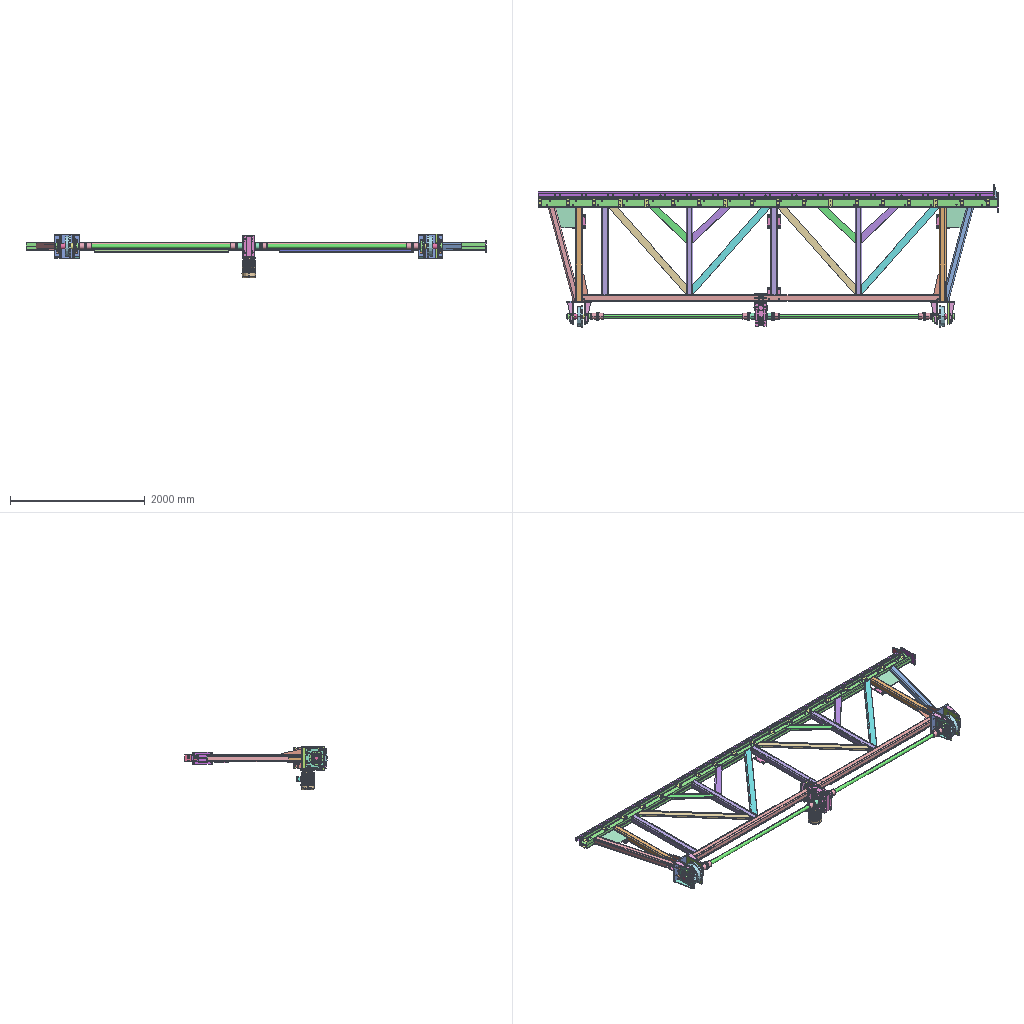Assembly | SolidWorks | 55 different items | 205 placed | box 6830 x 2120 x 652 mm
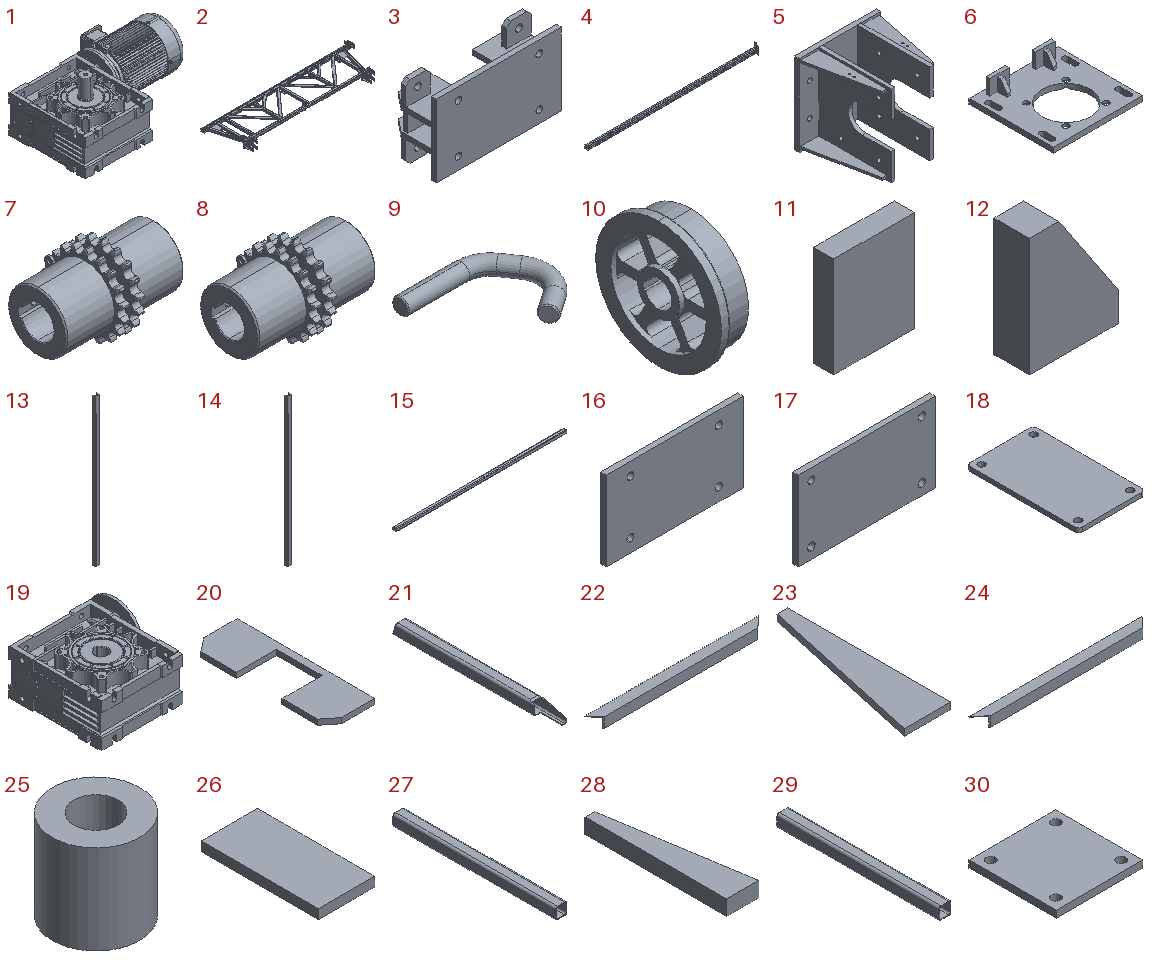Parts list (item | name | quantity | parent item | size | volume | features):
1 | (subassembly) | x1 | - | 618.25 x 437.5 x 340 mm | 18932676 mm3 | -
2 | (subassembly) | x1 | - | 6830 x 2073 x 360 mm | 92757683 mm3 | features ReferencePattern 15, LocalLPattern 6, MateUpdatePoint 2
3 | (subassembly) | x1 | - | 310 x 117 x 180 mm | 1412494 mm3 | features ReferencePattern 5, MirrorCompFeat 3, LocalLPattern 1
4 | (subassembly) | x1 | in 2 | 6830 x 180 x 420 mm | 27298052 mm3 | features ReferencePattern 33, LocalLPattern 3
5 | (subassembly) | x2 | in 2 | 360 x 340 x 360 mm | 6139471 mm3 | -
6 | (subassembly) | x4 | - | 280 x 265 x 64 mm | 917808 mm3 | features ReferencePattern 2, LocalLPattern 1
7 | (subassembly) | x2 | - | 178.9 x 120.134 x 117.94 mm | 791458 mm3 | features CompositeCurve 3
8 | (subassembly) | x2 | - | 178.9 x 120.134 x 117.94 mm | 822533 mm3 | features CompositeCurve 3
9 | - | x1 | - | 104.462 x 91.811 x 16 mm | 34123 mm3 | features Chamfer 2, WeldMemberFeat 1, WeldmentFeature 1
10 | - | x2 | - | 86 x 330 x 330 mm | 3397345 mm3 | features ICE 2, Revolution 1
11 | - | x8 | in 6 | 48 x 12 x 60 mm | 34560 mm3 | features Extrusion 1
12 | - | x8 | in 6 | 30 x 12 x 40 mm | 10800 mm3 | features Extrusion 1
13 | - | x1 | in 2 | 50 x 37 x 2000 mm | 1093372 mm3 | features Extrusion 1
14 | - | x1 | in 2 | 50 x 37 x 2000 mm | 1093372 mm3 | features Extrusion 1
15 | - | x1 | in 2 | 5300 x 100 x 100 mm | 11061763 mm3 | features LPattern 3, ICE 1, RefAxis 1, WeldMemberFeat 1, WeldmentFeature 1
16 | - | x1 | in 3 | 310 x 12 x 180 mm | 659949 mm3 | features Extrusion 1
17 | - | x1 | in 2 | 310 x 12 x 180 mm | 659016 mm3 | features Extrusion 1
18 | - | x1 | in 4 | 180 x 300 x 12 mm | 634755 mm3 | features Extrusion 1, ICE 1
19 | - | x1 | in 1 | 326.25 x 377.5 x 200 mm | 11644494 mm3 | features Boss 16, Cut 16, Fillet 5, CirPattern 3, Chamfer 2, Revolution 2, MirrorPattern 1
20 | - | x2 | in 3 | 105 x 310 x 12 mm | 271800 mm3 | features Extrusion 1, ICE 1
21 | - | x1 | in 2 | 100 x 1442 x 100 mm | 2662768 mm3 | features MirrorStock 1
22 | - | x2 | in 2 | 1732 x 100 x 100 mm | 1888735 mm3 | features Extrusion 1, ICE 1
23 | - | x6 | in 2 | 85 x 300 x 12 mm | 189000 mm3 | features Extrusion 1
24 | - | x2 | in 2 | 1732 x 100 x 100 mm | 1888735 mm3 | features Extrusion 1, ICE 1
25 | - | x8 | in 7, 8 | 11.91 x 11.91 x 12.2 mm | 1014 mm3 | features Extrusion 1
26 | - | x1 | in 4 | 96 x 200 x 16 mm | 307200 mm3 | features Extrusion 1
27 | - | x2 | in 2 | 100 x 1393 x 100 mm | 2912161 mm3 | features WeldMemberFeat 1, WeldmentFeature 1
28 | - | x3 | in 4 | 34 x 150 x 16 mm | 52800 mm3 | features Extrusion 1
29 | - | x4 | in 2 | 100 x 1293 x 100 mm | 2703104 mm3 | features WeldMemberFeat 1, WeldmentFeature 1
30 | - | x6 | in 2 | 200 x 200 x 16 mm | 617833 mm3 | features Extrusion 1, ICE 1, RefAxis 1
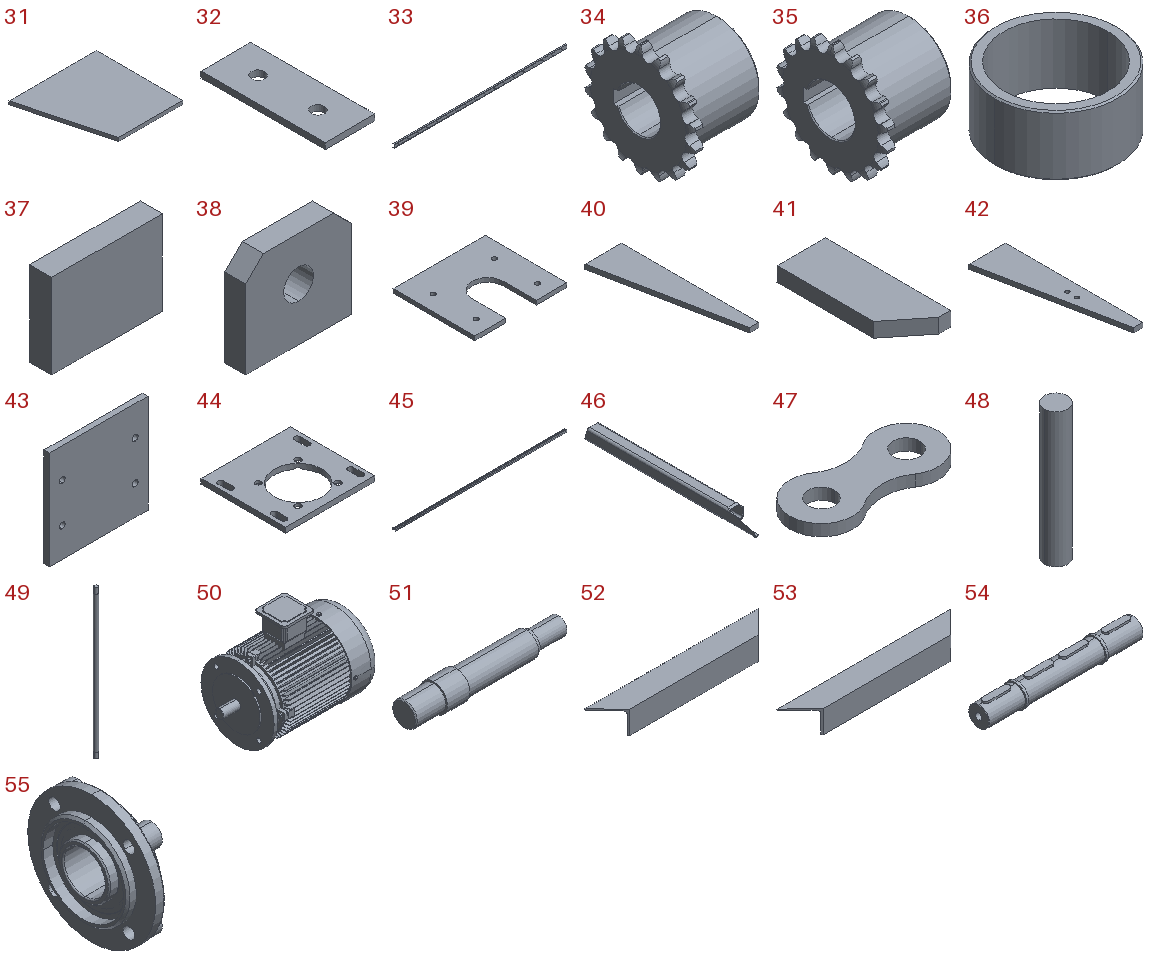31 | - | x2 | in 2 | 303 x 300 x 12 mm | 946107 mm3 | features Extrusion 1
32 | - | x36 | in 4 | 50 x 124 x 6 mm | 35607 mm3 | features Extrusion 1, ICE 1
33 | - | x2 | in 4 | 6818 x 58 x 140 mm | 12457918 mm3 | features ICE 2, LPattern 1, WeldMemberFeat 1, WeldmentFeature 1
34 | - | x2 | in 8 | 84 x 116.518 x 117.9 mm | 421510 mm3 | features ICE 2, Chamfer 1, CirPattern 1, HoleWzd 1, RefAxis 1, Revolution 1
35 | - | x6 | in 7, 8 | 84 x 116.558 x 117.94 mm | 390436 mm3 | features ICE 2, Chamfer 1, CirPattern 1, HoleWzd 1, RefAxis 1, Revolution 1
36 | - | x2 | - | 83 x 83 x 40.5 mm | 63009 mm3 | features Chamfer 1, Extrusion 1
37 | - | x2 | in 3 | 60 x 12 x 46 mm | 33120 mm3 | features Extrusion 1
38 | - | x4 | in 3 | 60 x 12 x 55 mm | 35676 mm3 | features Chamfer 1, Extrusion 1
39 | - | x4 | in 5 | 360 x 320 x 16 mm | 1488595 mm3 | features ICE 2, Extrusion 1, LPattern 1
40 | - | x4 | in 5 | 80 x 300 x 10 mm | 150000 mm3 | features Extrusion 1
41 | - | x2 | in 2 | 40 x 104 x 12 mm | 45600 mm3 | features ICE 2, Extrusion 1
42 | - | x4 | in 5 | 80 x 300 x 10 mm | 148995 mm3 | features Extrusion 1, ICE 1
43 | - | x2 | in 5 | 360 x 20 x 360 mm | 2564291 mm3 | features Extrusion 1, HoleWzd 1, LPattern 1
44 | - | x4 | in 6 | 280 x 265 x 16 mm | 827088 mm3 | features ICE 3, Extrusion 1
45 | - | x1 | - | 6768 x 93.66 x 93.66 mm | 19411583 mm3 | features ICE 1, WeldMemberFeat 1, WeldmentFeature 1
46 | - | x1 | in 2 | 100 x 1442 x 100 mm | 2662768 mm3 | features ICE 3, WeldMemberFeat 1, WeldmentFeature 1
47 | - | x32 | in 7, 8 | 33.05 x 14 x 2.55 mm | 777.67 mm3 | features Extrusion 1
48 | - | x4 | in 7, 8 | 8 x 8 x 46.5 mm | 2337 mm3 | features Extrusion 1
49 | - | x2 | - | 60 x 60 x 2235 mm | 6164294 mm3 | features ICE 2, Chamfer 1, Extrusion 1, MirrorPattern 1
50 | - | x1 | in 1 | 342 x 207 x 263.5 mm | 6736736 mm3 | features Boss 15, Cut 5, Revolution 5, Fillet 4, Chamfer 3, CirPattern 3, RevCut 2, 3DProfileFeature 1, MirrorPattern 1, MoveCopyBody 1
51 | - | x2 | - | 445 x 80 x 80 mm | 1605911 mm3 | features ICE 6, Chamfer 2, 3DProfileFeature 1, Extrusion 1, RefAxis 1
52 | - | x2 | in 2 | 761.728 x 100 x 100 mm | 732885 mm3 | features Extrusion 1, ICE 1
53 | - | x2 | in 2 | 761.728 x 100 x 100 mm | 732885 mm3 | features Extrusion 1, ICE 1
54 | - | x1 | in 1 | 340 x 51 x 51.5 mm | 551448 mm3 | features MirrorPattern 4, Chamfer 1, HoleWzd 1, ICE 1, Revolution 1
55 | - | x4 | - | 75.4 x 215 x 215 mm | 900645 mm3 | features BaseBody 1
Mates (type | each side: item.copy, entity, surface, feature):
In the top assembly
Coincident | 39.1 face plane Extrude1 | 44.1 face plane Extrude1
Coincident | 5.1 plane | 6.1 plane
DistanceDim | 39.1 face plane Extrude1 | 44.1 face plane Extrude5
Coincident | 44.1 face plane Extrude5 | 44.2 face plane Extrude5
Concentric | 44.1 face cylinder Extrude1 | 44.2 face cylinder Extrude1
Coincident | 39.2 face plane Extrude1 | 44.2 face plane Extrude1
Concentric | 44.1 face cylinder Extrude1 | 55.1 face cylinder snr_ucfc214_0
Coincident | 44.1 face plane Extrude1 | 55.1 face plane snr_ucfc214_0
Concentric | 44.1 face cylinder Extrude2 | 55.1 face cylinder snr_ucfc214_0
Concentric | 55.2 face cylinder snr_ucfc214_0 | 44.2 face cylinder Extrude1
Concentric | 44.2 face cylinder Extrude2 | 55.2 face cylinder snr_ucfc214_0
Coincident | 44.2 face plane Extrude1 | 55.2 face plane snr_ucfc214_0
Concentric | 51.1 face cylinder Extrude3 | 55.1 face cylinder snr_ucfc214_0
Coincident | 55.1 face plane snr_ucfc214_0 | 51.1 face plane Extrude1
Coincident | 51.1 face plane Extrude4 | assembly face
Parallel | assembly face | 10.1 face plane Extrude2
Concentric | 51.1 face cylinder Extrude2 | 10.1 face cylinder Revolve1
Coincident | 51.1 face plane Extrude1 | 10.1 face plane Revolve1
Concentric | 51.1 face cylinder Extrude2 | 36.1 face cylinder Extrude1
Coincident | 10.1 face plane Revolve1 | 36.1 face plane Extrude1
Concentric | 55.3 face cylinder snr_ucfc214_0 | 51.2 face cylinder Extrude3
Coincident | 55.3 face plane snr_ucfc214_0 | 51.2 face plane Extrude1
Coincident | 51.2 face plane Extrude4 | assembly face
Concentric | 51.2 face cylinder Extrude4 | assembly face | 2 times
Parallel | assembly face | 10.2 face plane Extrude2
Concentric | 51.2 face cylinder Extrude2 | 10.2 face cylinder Revolve1
Coincident | 51.2 face plane Extrude1 | 10.2 face plane Revolve1
Concentric | 51.2 face cylinder Extrude6 | 36.2 face cylinder Extrude1
Coincident | 10.2 face plane Revolve1 | 36.2 face plane Extrude1
Coincident | 45.1 face plane Structural Member1 | 26.1 face plane Extrude1
Coincident | 33.1 face plane Structural Member1 | 45.1 face plane Structural Member1
Coincident | 33.2 edge | 45.1 edge
Concentric | 45.1 face cylinder Extrude1 | assembly face | 4 times
Tangent | 33.1 face cylinder Structural Member1 | assembly face
Parallel | 45.1 face plane Structural Member1 | assembly plane
Coincident | 45.1 face plane Structural Member1 | assembly face | 2 times
Coincident | assembly face | assembly face
Concentric | assembly face | 45.1 face cylinder Extrude1
Parallel | assembly plane | assembly plane
Tangent | 33.2 face cylinder Structural Member1 | assembly face
Parallel | 39.3 face plane Extrude1 | assembly face
Parallel | 39.2 face plane Extrude1 | assembly face
Concentric | 51.1 face cylinder Extrude4 | assembly face
DistanceDim | 15.1 face plane Structural Member1 | 20.1 face plane Extrude1
Concentric | 17.1 face cylinder Extrude1 | 38.1 face cylinder Boss-Extrude1
Concentric | 17.1 face cylinder Extrude1 | 38.2 face cylinder Boss-Extrude1
Coincident | 16.1 face plane Extrude1 | 19.1 face plane Extrude15
Concentric | 51.1 face cylinder Extrude6 | 49.1 face cylinder Extrude1
DistanceDim | 51.1 face plane Extrude6 | 49.1 face plane Extrude2
Concentric | 49.1 face cylinder Extrude1 | 35.1 face cylinder Revolve1
Coincident | 49.1 face plane Extrude2 | 35.2 face plane Revolve1
Coincident | 38.3 face plane Boss-Extrude1 | assembly face
Coincident | 49.1 face plane Extrude1 | 35.3 face plane Revolve1
Concentric | 16.1 face cylinder Extrude1 | 19.1 face cylinder Cut-Extrude8 | 2 times
Concentric | 49.1 face cylinder Mirror1 | 35.3 face cylinder Revolve1
In subassembly 2
Coincident | 15.2 face plane Structural Member1 | 27.1 face plane Structural Member1 | 3 times
Coincident | 43.1 face plane Extrude1 | 27.1 face plane Structural Member1
DistanceDim | 43.1 face plane Extrude1 | 27.1 face plane Structural Member1 | 2 times
Coincident | 15.2 face plane Structural Member1 | 29.1 face plane Structural Member1 | 2 times
DistanceDim | 15.2 plane | 29.1 face plane Structural Member1
Coincident | 27.2 plane | 33.3 face plane Structural Member1
Coincident | 27.2 face plane Structural Member1 | 33.3 face plane Structural Member1
Coincident | 33.3 face plane Structural Member1 | 31.1 face plane Extrude1
Coincident | 27.1 face plane Structural Member1 | 31.1 face plane Extrude1
Coincident | 27.1 face plane Structural Member1 | 23.1 face plane Extrude1 | 2 times
Coincident | 43.1 face plane Extrude1 | 23.1 face plane Extrude1
Coincident | 33.4 edge | 31.1 face plane Extrude1
DistanceDim | 13.1 face plane Extrude1 | 29.1 face plane Structural Member1
DistanceDim | 13.1 face plane Extrude1 | 15.2 face plane Structural Member1
Coincident | 15.2 face plane Structural Member1 | 13.1 edge
Coincident | 14.1 face plane Extrude1 | 13.1 face plane Extrude1 | 2 times
Coincident | 27.2 face plane Structural Member1 | 30.1 face plane Extrude1
Concentric | 15.2 face cylinder LPattern3 | 30.1 face cylinder Extrude2
Coincident | 15.2 face plane Structural Member1 | 29.2 face plane Structural Member1 | 2 times
DistanceDim | 29.1 face plane Structural Member1 | 29.2 face plane Structural Member1
Coincident | 29.2 face plane Structural Member1 | 22.1 face plane Extrude1
Coincident | 29.2 face plane Structural Member1 | 22.1 face plane Extrude2
Coincident | 33.3 face plane Structural Member1 | 22.1 face plane Extrude2
Coincident | 29.2 face plane Structural Member1 | 24.1 face plane Extrude5
Coincident | 22.1 face plane Extrude1 | 24.1 face plane Extrude1
Coincident | 33.3 face plane Structural Member1 | 24.1 face plane Extrude5
Coincident | 29.2 face plane Structural Member1 | 53.1 face plane Extrude5
Coincident | 22.1 face plane Extrude1 | 53.1 face plane Extrude1
Coincident | 33.3 face plane Structural Member1 | 53.1 edge
Coincident | 29.2 face plane Structural Member1 | 52.1 face plane Extrude5
Coincident | 29.2 face plane Structural Member1 | 52.1 face plane Extrude1
Coincident | 33.3 face plane Structural Member1 | 52.1 edge
Coincident | 29.3 face plane Structural Member1 | 29.4 face plane Structural Member1
Coincident | 15.2 face plane Structural Member1 | 29.4 face plane Structural Member1
DistanceDim | 29.4 face plane Structural Member1 | 27.1 face plane Structural Member1
DistanceDim | 27.1 face plane Structural Member1 | 33.3 face plane Structural Member1
Coincident | 27.1 face plane Structural Member1 | 23.2 face plane Extrude1
Coincident | 15.2 face plane Structural Member1 | 23.2 face plane Extrude1
Coincident | 31.1 face plane Extrude1 | 23.2 face plane Extrude1
Coincident | 27.1 face plane Structural Member1 | 46.1 face plane Cut-Extrude1
Coincident | 27.1 face plane Structural Member1 | 46.1 face plane Structural Member1
Coincident | 43.1 face plane Extrude1 | 46.1 edge
Coincident | 27.2 face plane Structural Member1 | 31.2 face plane Extrude1
Coincident | 33.4 face plane Structural Member1 | 31.2 face plane Extrude1
Coincident | 31.1 face plane Extrude1 | 31.2 face plane Extrude1
Coincident | 27.2 face plane Structural Member1 | 21.1 face plane Side Diagonal Column10 Meter Width Minus FourMirror | 2 times
Coincident | 27.2 face plane Structural Member1 | 23.3 face plane Extrude1
Coincident | 15.2 face plane Structural Member1 | 23.3 face plane Extrude1
Coincident | 31.2 face plane Extrude1 | 23.3 face plane Extrude1
Coincident | 43.2 face plane Extrude1 | 21.1 edge
Coincident | 43.2 face plane Extrude1 | 27.2 face plane Structural Member1
Coincident | 15.2 face plane Structural Member1 | 17.2 face plane Extrude1
Coincident | 15.2 face plane Structural Member1 | 41.1 face plane Extrude3
Coincident | 41.1 face plane Cut-Extrude1 | 17.2 face plane Extrude1
DistanceDim | 41.1 face plane Extrude1 | 17.2 face plane Extrude1
DistanceDim | 17.2 face plane Extrude1 | 29.1 face plane Structural Member1
DistanceDim | 17.2 face plane Extrude1 | 15.2 face plane Structural Member1
Coincident | 15.2 face plane Structural Member1 | 41.2 face plane Extrude3
Coincident | 17.2 face plane Extrude1 | 41.2 face plane Cut-Extrude1
Coincident | 41.1 face plane Extrude1 | 41.2 face plane Extrude1
In subassembly 4
Coincident | 33.5 face plane Structural Member1 | 33.6 face plane Structural Member1 | 3 times
Coincident | 33.5 plane | 26.2 plane
Coincident | 33.5 face plane Structural Member1 | 26.2 face plane Extrude1
Coincident | 33.5 face plane Structural Member1 | 26.2 plane
Coincident | 26.2 plane | 28.1 plane
Coincident | 33.6 face plane Structural Member1 | 28.1 face plane Extrude1
Coincident | 26.2 face plane Extrude1 | 28.1 face plane Extrude1
Coincident | 28.2 plane | 26.2 plane
Coincident | 28.2 face plane Extrude1 | 33.6 face plane Structural Member1
Coincident | 28.2 face plane Extrude1 | 26.2 face plane Extrude1
Coincident | 33.6 plane | 32.1 face plane Extrude1
Coincident | 33.6 face cylinder Structural Member1 | 32.1 edge
Coincident | 33.5 plane | 32.2 face plane Extrude1
Coincident | 33.5 face cylinder Structural Member1 | 32.2 edge
Coincident | 33.5 plane | 32.3 face plane Extrude1
Coincident | 33.5 face plane Structural Member1 | 32.3 face plane Extrude1
Coincident | 33.5 face cylinder Structural Member1 | 32.3 edge
Coincident | 32.4 face plane Extrude1 | 33.6 plane
Coincident | 33.6 face plane Structural Member1 | 32.4 face plane Extrude1
Coincident | 33.6 face cylinder Structural Member1 | 32.4 edge
DistanceDim | 32.2 face plane Extrude1 | 33.5 face plane Structural Member1
Coincident | 32.1 face plane Extrude1 | 32.2 face plane Extrude1
Coincident | 33.6 face plane Structural Member1 | 18.1 face plane Extrude1
Coincident | 33.6 plane | 18.1 plane
Coincident | 33.6 face plane Structural Member1 | 18.1 plane
In subassembly 5
Coincident | 43.3 face plane Extrude1 | 39.4 face plane Extrude1 | 2 times
Symmetric | 43.3 plane | 39.5 face plane Extrude1 | 39.4 face plane Extrude1
Coincident | 43.3 face plane Extrude1 | 39.5 face plane Extrude1 | 2 times
DistanceDim | 39.4 face plane Extrude1 | 39.5 face plane Extrude1
Coincident | 42.1 face plane Extrude1 | 39.4 face plane Extrude1
DistanceDim | 42.1 face plane Extrude1 | 39.4 face plane Extrude1
Coincident | 43.3 face plane Extrude1 | 42.1 face plane Extrude1
Coincident | 39.5 face plane Extrude1 | 42.2 face plane Extrude1
DistanceDim | 42.2 face plane Extrude1 | 39.5 face plane Extrude1
Coincident | 43.3 face plane Extrude1 | 42.2 face plane Extrude1
Coincident | 40.1 face plane Extrude1 | 39.4 face plane Extrude1
DistanceDim | 42.1 face plane Extrude1 | 40.1 face plane Extrude1
Coincident | 43.3 face plane Extrude1 | 40.1 face plane Extrude1
DistanceDim | 40.2 face plane Extrude1 | 42.2 face plane Extrude1
Coincident | 43.3 face plane Extrude1 | 40.2 edge
Coincident | 39.5 face plane Extrude1 | 40.2 face plane Extrude1
In subassembly 6
DistanceDim | 11.1 face plane Extrude1 | 44.3 face plane Extrude1 | 2 times
Coincident | 44.3 face plane Extrude1 | 11.1 face plane Extrude1
Coincident | 11.1 face plane Extrude1 | 12.1 face plane Extrude1
Coincident | 44.3 face plane Extrude1 | 12.1 edge
Coincident | 11.1 plane | 12.1 plane
In subassembly 3
Coincident | 16.2 face plane Extrude1 | 20.2 face plane Extrude1 | 2 times
DistanceDim | 20.2 face plane Extrude1 | 16.2 face plane Extrude1
Coincident | 20.3 face plane Extrude1 | 38.4 face plane Boss-Extrude1 | 2 times
DistanceDim | 38.4 face plane Boss-Extrude1 | 20.3 face plane Extrude3
Coincident | 38.4 face plane Boss-Extrude1 | 37.1 face plane Boss-Extrude1
Coincident | 20.3 face plane Extrude1 | 37.1 face plane Boss-Extrude1
DistanceDim | 37.1 face plane Boss-Extrude1 | 20.3 face plane Extrude1
In subassembly 1
Coincident | 19.2 face plane Revolve5 | 50.1 face plane Revolve1
Concentric | 19.2 face cylinder Revolve5 | 50.1 face cylinder Revolve1
Concentric | 50.1 face cylinder CirPattern9 | 19.2 face cylinder Cut-Extrude13
Coincident | 19.2 face plane Revolve6 | 54.1 face plane Revolve1
Concentric | 19.2 face cylinder Revolve6 | 54.1 face cylinder Revolve1
Coincident | 19.2 face plane Cut-Extrude11 | 54.1 face plane Mirror1
In subassembly 8
DistanceDim | 34.1 face plane Revolve1 | 35.4 face plane Revolve1
Concentric | 35.4 face cylinder Revolve1 | 34.1 face cylinder Revolve1
Coincident | 35.4 plane | 34.1 plane
Concentric | 47.1 face cylinder Boss-Extrude1 | 47.2 face cylinder Boss-Extrude1
Coincident | 47.1 face plane Boss-Extrude1 | 47.2 face plane Boss-Extrude1
Concentric | 25.1 face cylinder Boss-Extrude1 | 47.1 edge
Coincident | 25.1 face plane Boss-Extrude1 | 47.1 face plane Boss-Extrude1
Coincident | 25.1 face plane Boss-Extrude1 | 47.3 face plane Boss-Extrude1
Concentric | 25.1 face cylinder Boss-Extrude1 | 47.4 edge
Concentric | 47.2 face cylinder Boss-Extrude1 | 47.4 face cylinder Boss-Extrude1
Coincident | 47.5 face plane Boss-Extrude1 | 47.4 face plane Boss-Extrude1
Concentric | 47.5 face cylinder Boss-Extrude1 | 47.4 face cylinder Boss-Extrude1
Coincident | 47.5 edge | 47.4 face cylinder Boss-Extrude1
Coincident | 47.6 face plane Boss-Extrude1 | 25.2 face plane Boss-Extrude1
Concentric | 47.5 face cylinder Boss-Extrude1 | 25.2 face cylinder Boss-Extrude1
Coincident | 47.4 face plane Boss-Extrude1 | 47.3 face plane Boss-Extrude1
Concentric | 47.4 face cylinder Boss-Extrude1 | 47.3 face cylinder Boss-Extrude1
Concentric | 47.1 face cylinder Boss-Extrude1 | 47.3 face cylinder Boss-Extrude1
Coincident | 47.5 face plane Boss-Extrude1 | 47.6 face plane Boss-Extrude1
Concentric | 47.5 face cylinder Boss-Extrude1 | 47.6 face cylinder Boss-Extrude1
Coincident | 25.2 face plane Boss-Extrude1 | 47.7 face plane Boss-Extrude1
Concentric | 25.2 face cylinder Boss-Extrude1 | 47.7 face cylinder Boss-Extrude1
Concentric | 47.6 face cylinder Boss-Extrude1 | 47.7 face cylinder Boss-Extrude1
Coincident | 47.7 face plane Boss-Extrude1 | 47.8 face plane Boss-Extrude1
Concentric | 47.5 face cylinder Boss-Extrude1 | 47.8 face cylinder Boss-Extrude1
Concentric | 47.7 face cylinder Boss-Extrude1 | 47.8 face cylinder Boss-Extrude1
Concentric | 47.8 face cylinder Boss-Extrude1 | 48.1 face cylinder Boss-Extrude1
DistanceDim | 48.1 face plane Boss-Extrude1 | 47.2 face plane Boss-Extrude1
Concentric | 34.1 face cylinder CirPattern1 | 47.7 face cylinder Boss-Extrude1
Concentric | 47.3 face cylinder Boss-Extrude1 | 8.1 face
Concentric | 34.1 face cylinder Cut-Extrude3 | 25.2 face cylinder Boss-Extrude1
DistanceDim | 47.6 face plane Boss-Extrude1 | 34.1 face plane Revolve1
In subassembly 7
Concentric | 47.1 face cylinder Boss-Extrude1 | 47.2 face cylinder Boss-Extrude1
Coincident | 47.1 face plane Boss-Extrude1 | 47.2 face plane Boss-Extrude1
Concentric | 25.1 face cylinder Boss-Extrude1 | 47.1 edge
Coincident | 25.1 face plane Boss-Extrude1 | 47.1 face plane Boss-Extrude1
Coincident | 25.1 face plane Boss-Extrude1 | 47.3 face plane Boss-Extrude1
Concentric | 25.1 face cylinder Boss-Extrude1 | 47.4 edge
Concentric | 47.2 face cylinder Boss-Extrude1 | 47.4 face cylinder Boss-Extrude1
Coincident | 47.5 face plane Boss-Extrude1 | 47.4 face plane Boss-Extrude1
Concentric | 47.5 face cylinder Boss-Extrude1 | 47.4 face cylinder Boss-Extrude1
Coincident | 47.5 edge | 47.4 face cylinder Boss-Extrude1
Coincident | 47.6 face plane Boss-Extrude1 | 25.2 face plane Boss-Extrude1
Concentric | 47.5 face cylinder Boss-Extrude1 | 25.2 face cylinder Boss-Extrude1
Coincident | 47.4 face plane Boss-Extrude1 | 47.3 face plane Boss-Extrude1
Concentric | 47.4 face cylinder Boss-Extrude1 | 47.3 face cylinder Boss-Extrude1
Concentric | 47.1 face cylinder Boss-Extrude1 | 47.3 face cylinder Boss-Extrude1
Coincident | 47.5 face plane Boss-Extrude1 | 47.6 face plane Boss-Extrude1
Concentric | 47.5 face cylinder Boss-Extrude1 | 47.6 face cylinder Boss-Extrude1
Coincident | 25.2 face plane Boss-Extrude1 | 47.7 face plane Boss-Extrude1
Concentric | 25.2 face cylinder Boss-Extrude1 | 47.7 face cylinder Boss-Extrude1
Concentric | 47.6 face cylinder Boss-Extrude1 | 47.7 face cylinder Boss-Extrude1
Coincident | 47.7 face plane Boss-Extrude1 | 47.8 face plane Boss-Extrude1
Concentric | 47.5 face cylinder Boss-Extrude1 | 47.8 face cylinder Boss-Extrude1
Concentric | 47.7 face cylinder Boss-Extrude1 | 47.8 face cylinder Boss-Extrude1
Concentric | 47.8 face cylinder Boss-Extrude1 | 48.1 face cylinder Boss-Extrude1
DistanceDim | 48.1 face plane Boss-Extrude1 | 47.2 face plane Boss-Extrude1
Concentric | 47.3 face cylinder Boss-Extrude1 | 7.1 face
Concentric | 35.4 face cylinder Revolve1 | 35.5 face cylinder Revolve1
Concentric | 35.4 face cylinder Cut-Extrude1 | 35.5 face cylinder Cut-Extrude1
Concentric | 35.4 face cylinder Cut-Extrude1 | 25.1 face cylinder Boss-Extrude1
DistanceDim | 35.5 face plane Revolve1 | 35.4 face plane Revolve1
DistanceDim | 47.6 face plane Boss-Extrude1 | 35.5 face plane Revolve1